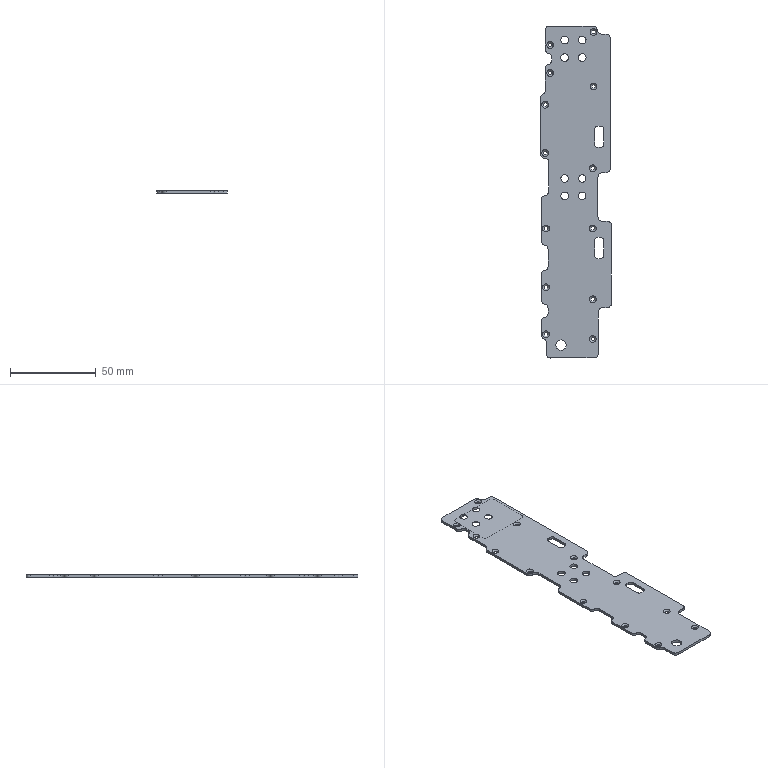Part | STEP file | Final stage amplifier cavity inner cover | 1 solid | 130 faces | box 41.47 x 194.01 x 1.5 mm | volume 9143 mm3 | cylinder 66 | plane 38 | cone 26 | commonest cylinder face diameters 5 x32 2.2 x13 4 x12 4.5 x8 6 x1